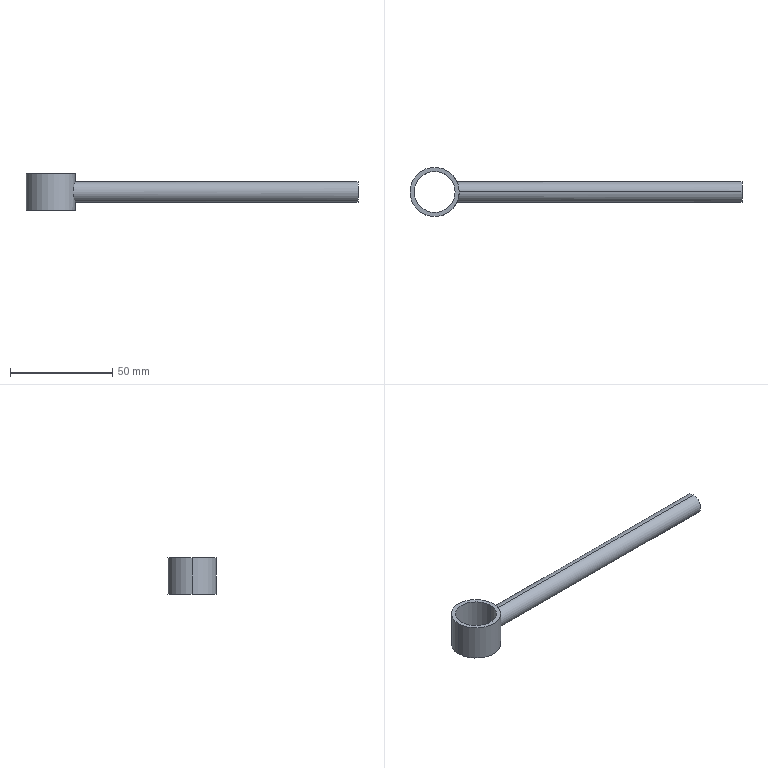Part | SolidWorks | features Extrusion 1, ICE 1 | 1 solid | 9 faces | box 162 x 24 x 18 mm | volume 13348 mm3 | cylinder 6 | plane 3 | commonest cylinder face diameters 10 x2 20 x2 24 x2
STEP:
#1=CARTESIAN_POINT('',(12.,0.,-5.));
#2=VERTEX_POINT('',#1);
#3=CARTESIAN_POINT('',(12.,0.,5.));
#4=VERTEX_POINT('',#3);
#5=CARTESIAN_POINT('',(12.,0.,-5.));
#6=CARTESIAN_POINT('',(12.,0.3345,-5.));
#7=CARTESIAN_POINT('',(11.986,0.6627,-4.967));
#8=CARTESIAN_POINT('',(11.933,1.307,-4.837));
#9=CARTESIAN_POINT('',(11.893,1.627,-4.739));
#10=CARTESIAN_POINT('',(11.795,2.231,-4.487));
#11=CARTESIAN_POINT('',(11.736,2.517,-4.333));
#12=CARTESIAN_POINT('',(11.607,3.058,-3.969));
#13=CARTESIAN_POINT('',(11.537,3.31,-3.761));
#14=CARTESIAN_POINT('',(11.396,3.766,-3.305));
#15=CARTESIAN_POINT('',(11.325,3.972,-3.055));
#16=CARTESIAN_POINT('',(11.191,4.335,-2.512));
#17=CARTESIAN_POINT('',(11.13,4.489,-2.227));
#18=CARTESIAN_POINT('',(11.051,4.677,-1.777));
#19=CARTESIAN_POINT('',(11.028,4.732,-1.623));
#20=CARTESIAN_POINT('',(10.986,4.829,-1.308));
#21=CARTESIAN_POINT('',(10.968,4.87,-1.146));
#22=CARTESIAN_POINT('',(10.924,4.967,-0.6608));
#23=CARTESIAN_POINT('',(10.909,5.,-0.3338));
#24=CARTESIAN_POINT('',(10.909,5.,0.3273));
#25=CARTESIAN_POINT('',(10.924,4.967,0.6627));
#26=CARTESIAN_POINT('',(10.982,4.837,1.308));
#27=CARTESIAN_POINT('',(11.025,4.741,1.622));
#28=CARTESIAN_POINT('',(11.13,4.487,2.231));
#29=CARTESIAN_POINT('',(11.192,4.333,2.516));
#30=CARTESIAN_POINT('',(11.325,3.972,3.054));
#31=CARTESIAN_POINT('',(11.397,3.763,3.308));
#32=CARTESIAN_POINT('',(11.538,3.306,3.765));
#33=CARTESIAN_POINT('',(11.607,3.057,3.97));
#34=CARTESIAN_POINT('',(11.704,2.652,4.242));
#35=CARTESIAN_POINT('',(11.735,2.51,4.327));
#36=CARTESIAN_POINT('',(11.793,2.222,4.482));
#37=CARTESIAN_POINT('',(11.82,2.075,4.552));
#38=CARTESIAN_POINT('',(11.893,1.625,4.74));
#39=CARTESIAN_POINT('',(11.933,1.312,4.836));
#40=CARTESIAN_POINT('',(11.986,0.659,4.968));
#41=CARTESIAN_POINT('',(12.,0.3295,5.));
#42=CARTESIAN_POINT('',(12.,0.,5.));
#43=B_SPLINE_CURVE_WITH_KNOTS('',3,(#5,#6,#7,#8,#9,#10,#11,#12,#13,#14,#15,#16,#17,#18,#19,#20,#21,#22,#23,#24,#25,#26,#27,#28,#29,#30,#31,#32,#33,#34,#35,#36,#37,#38,#39,#40,#41,#42),.UNSPECIFIED.,.F.,.F.,(4,2,2,2,2,2,2,2,2,2,2,2,2,2,2,2,2,2,4),(0.,0.0009884,0.001977,0.002965,0.003954,0.004942,0.005931,0.006425,0.006919,0.007907,0.008896,0.009884,0.01087,0.01186,0.01285,0.01334,0.01384,0.01483,0.01581),.UNSPECIFIED.);
#44=EDGE_CURVE('',#2,#4,#43,.T.);
#45=ORIENTED_EDGE('',*,*,#44,.T.);
#46=CARTESIAN_POINT('',(150.,0.,5.));
#47=VERTEX_POINT('',#46);
#48=CARTESIAN_POINT('',(-12.002,0.,5.));
#49=DIRECTION('',(1.,0.,0.));
#50=VECTOR('',#49,1000.);
#51=LINE('',#48,#50);
#52=EDGE_CURVE('',#4,#47,#51,.T.);
#53=ORIENTED_EDGE('',*,*,#52,.T.);
#54=CARTESIAN_POINT('',(150.,0.,-5.));
#55=VERTEX_POINT('',#54);
#56=CARTESIAN_POINT('',(150.,0.,0.));
#57=DIRECTION('',(1.,0.,0.));
#58=DIRECTION('',(0.,0.,-1.));
#59=AXIS2_PLACEMENT_3D('',#56,#57,#58);
#60=CIRCLE('',#59,5.);
#61=EDGE_CURVE('',#55,#47,#60,.T.);
#62=ORIENTED_EDGE('',*,*,#61,.F.);
#63=CARTESIAN_POINT('',(-12.002,0.,-5.));
#64=DIRECTION('',(1.,0.,0.));
#65=VECTOR('',#64,1000.);
#66=LINE('',#63,#65);
#67=EDGE_CURVE('',#2,#55,#66,.T.);
#68=ORIENTED_EDGE('',*,*,#67,.F.);
#69=EDGE_LOOP('',(#45,#53,#62,#68));
#70=FACE_OUTER_BOUND('',#69,.T.);
#71=CARTESIAN_POINT('',(-12.002,0.,0.));
#72=DIRECTION('',(1.,0.,0.));
#73=DIRECTION('',(0.,0.,-1.));
#74=AXIS2_PLACEMENT_3D('',#71,#72,#73);
#75=CYLINDRICAL_SURFACE('',#74,5.);
#76=ADVANCED_FACE('',(#70),#75,.T.);
#77=CARTESIAN_POINT('',(-10.,0.,9.));
#78=VERTEX_POINT('',#77);
#79=CARTESIAN_POINT('',(10.,0.,9.));
#80=VERTEX_POINT('',#79);
#81=CARTESIAN_POINT('',(0.,0.,9.));
#82=DIRECTION('',(0.,0.,1.));
#83=DIRECTION('',(1.,0.,0.));
#84=AXIS2_PLACEMENT_3D('',#81,#82,#83);
#85=CIRCLE('',#84,10.);
#86=EDGE_CURVE('',#78,#80,#85,.T.);
#87=ORIENTED_EDGE('',*,*,#86,.T.);
#88=CARTESIAN_POINT('',(10.,0.,-9.));
#89=VERTEX_POINT('',#88);
#90=CARTESIAN_POINT('',(10.,0.,9.));
#91=DIRECTION('',(0.,0.,-1.));
#92=VECTOR('',#91,1000.);
#93=LINE('',#90,#92);
#94=EDGE_CURVE('',#80,#89,#93,.T.);
#95=ORIENTED_EDGE('',*,*,#94,.T.);
#96=CARTESIAN_POINT('',(-10.,0.,-9.));
#97=VERTEX_POINT('',#96);
#98=CARTESIAN_POINT('',(0.,0.,-9.));
#99=DIRECTION('',(0.,0.,1.));
#100=DIRECTION('',(1.,0.,0.));
#101=AXIS2_PLACEMENT_3D('',#98,#99,#100);
#102=CIRCLE('',#101,10.);
#103=EDGE_CURVE('',#97,#89,#102,.T.);
#104=ORIENTED_EDGE('',*,*,#103,.F.);
#105=CARTESIAN_POINT('',(-10.,0.,9.));
#106=DIRECTION('',(0.,0.,-1.));
#107=VECTOR('',#106,1000.);
#108=LINE('',#105,#107);
#109=EDGE_CURVE('',#78,#97,#108,.T.);
#110=ORIENTED_EDGE('',*,*,#109,.F.);
#111=EDGE_LOOP('',(#87,#95,#104,#110));
#112=FACE_OUTER_BOUND('',#111,.T.);
#113=CARTESIAN_POINT('',(0.,0.,9.));
#114=DIRECTION('',(0.,0.,-1.));
#115=DIRECTION('',(-1.,0.,0.));
#116=AXIS2_PLACEMENT_3D('',#113,#114,#115);
#117=CYLINDRICAL_SURFACE('',#116,10.);
#118=ADVANCED_FACE('',(#112),#117,.F.);
#119=CARTESIAN_POINT('',(12.,0.,9.));
#120=VERTEX_POINT('',#119);
#121=CARTESIAN_POINT('',(-12.,0.,9.));
#122=VERTEX_POINT('',#121);
#123=CARTESIAN_POINT('',(0.,0.,9.));
#124=DIRECTION('',(0.,0.,1.));
#125=DIRECTION('',(1.,0.,0.));
#126=AXIS2_PLACEMENT_3D('',#123,#124,#125);
#127=CIRCLE('',#126,12.);
#128=EDGE_CURVE('',#120,#122,#127,.T.);
#129=ORIENTED_EDGE('',*,*,#128,.F.);
#130=CARTESIAN_POINT('',(12.,0.,9.));
#131=DIRECTION('',(0.,0.,-1.));
#132=VECTOR('',#131,1000.);
#133=LINE('',#130,#132);
#134=EDGE_CURVE('',#120,#4,#133,.T.);
#135=ORIENTED_EDGE('',*,*,#134,.T.);
#136=ORIENTED_EDGE('',*,*,#44,.F.);
#137=CARTESIAN_POINT('',(12.,0.,-9.));
#138=VERTEX_POINT('',#137);
#139=CARTESIAN_POINT('',(12.,0.,9.));
#140=DIRECTION('',(0.,0.,-1.));
#141=VECTOR('',#140,1000.);
#142=LINE('',#139,#141);
#143=EDGE_CURVE('',#2,#138,#142,.T.);
#144=ORIENTED_EDGE('',*,*,#143,.T.);
#145=CARTESIAN_POINT('',(-12.,0.,-9.));
#146=VERTEX_POINT('',#145);
#147=CARTESIAN_POINT('',(0.,0.,-9.));
#148=DIRECTION('',(0.,0.,1.));
#149=DIRECTION('',(1.,0.,0.));
#150=AXIS2_PLACEMENT_3D('',#147,#148,#149);
#151=CIRCLE('',#150,12.);
#152=EDGE_CURVE('',#138,#146,#151,.T.);
#153=ORIENTED_EDGE('',*,*,#152,.T.);
#154=CARTESIAN_POINT('',(-12.,0.,9.));
#155=DIRECTION('',(0.,0.,-1.));
#156=VECTOR('',#155,1000.);
#157=LINE('',#154,#156);
#158=EDGE_CURVE('',#122,#146,#157,.T.);
#159=ORIENTED_EDGE('',*,*,#158,.F.);
#160=EDGE_LOOP('',(#129,#135,#136,#144,#153,#159));
#161=FACE_OUTER_BOUND('',#160,.T.);
#162=CARTESIAN_POINT('',(0.,0.,9.));
#163=DIRECTION('',(0.,0.,-1.));
#164=DIRECTION('',(-1.,0.,0.));
#165=AXIS2_PLACEMENT_3D('',#162,#163,#164);
#166=CYLINDRICAL_SURFACE('',#165,12.);
#167=ADVANCED_FACE('',(#161),#166,.T.);
#168=CARTESIAN_POINT('',(0.,0.,9.));
#169=DIRECTION('',(0.,0.,1.));
#170=DIRECTION('',(1.,0.,0.));
#171=AXIS2_PLACEMENT_3D('',#168,#169,#170);
#172=CIRCLE('',#171,12.);
#173=EDGE_CURVE('',#122,#120,#172,.T.);
#174=ORIENTED_EDGE('',*,*,#173,.T.);
#175=ORIENTED_EDGE('',*,*,#128,.T.);
#176=EDGE_LOOP('',(#174,#175));
#177=FACE_OUTER_BOUND('',#176,.T.);
#178=ORIENTED_EDGE('',*,*,#86,.F.);
#179=CARTESIAN_POINT('',(0.,0.,9.));
#180=DIRECTION('',(0.,0.,1.));
#181=DIRECTION('',(1.,0.,0.));
#182=AXIS2_PLACEMENT_3D('',#179,#180,#181);
#183=CIRCLE('',#182,10.);
#184=EDGE_CURVE('',#80,#78,#183,.T.);
#185=ORIENTED_EDGE('',*,*,#184,.F.);
#186=EDGE_LOOP('',(#178,#185));
#187=FACE_BOUND('',#186,.T.);
#188=CARTESIAN_POINT('',(0.,0.,9.));
#189=DIRECTION('',(0.,0.,1.));
#190=DIRECTION('',(1.,0.,0.));
#191=AXIS2_PLACEMENT_3D('',#188,#189,#190);
#192=PLANE('',#191);
#193=ADVANCED_FACE('',(#177,#187),#192,.T.);
#194=CARTESIAN_POINT('',(0.,0.,-9.));
#195=DIRECTION('',(0.,0.,1.));
#196=DIRECTION('',(1.,0.,0.));
#197=AXIS2_PLACEMENT_3D('',#194,#195,#196);
#198=CIRCLE('',#197,12.);
#199=EDGE_CURVE('',#146,#138,#198,.T.);
#200=ORIENTED_EDGE('',*,*,#199,.F.);
#201=ORIENTED_EDGE('',*,*,#152,.F.);
#202=EDGE_LOOP('',(#200,#201));
#203=FACE_OUTER_BOUND('',#202,.T.);
#204=ORIENTED_EDGE('',*,*,#103,.T.);
#205=CARTESIAN_POINT('',(0.,0.,-9.));
#206=DIRECTION('',(0.,0.,1.));
#207=DIRECTION('',(1.,0.,0.));
#208=AXIS2_PLACEMENT_3D('',#205,#206,#207);
#209=CIRCLE('',#208,10.);
#210=EDGE_CURVE('',#89,#97,#209,.T.);
#211=ORIENTED_EDGE('',*,*,#210,.T.);
#212=EDGE_LOOP('',(#204,#211));
#213=FACE_BOUND('',#212,.T.);
#214=CARTESIAN_POINT('',(0.,0.,-9.));
#215=DIRECTION('',(0.,0.,1.));
#216=DIRECTION('',(1.,0.,0.));
#217=AXIS2_PLACEMENT_3D('',#214,#215,#216);
#218=PLANE('',#217);
#219=ADVANCED_FACE('',(#203,#213),#218,.F.);
#220=ORIENTED_EDGE('',*,*,#134,.F.);
#221=ORIENTED_EDGE('',*,*,#173,.F.);
#222=ORIENTED_EDGE('',*,*,#158,.T.);
#223=ORIENTED_EDGE('',*,*,#199,.T.);
#224=ORIENTED_EDGE('',*,*,#143,.F.);
#225=CARTESIAN_POINT('',(12.,0.,5.));
#226=CARTESIAN_POINT('',(12.,-0.1646,5.));
#227=CARTESIAN_POINT('',(11.997,-0.3295,4.992));
#228=CARTESIAN_POINT('',(11.983,-0.6596,4.959));
#229=CARTESIAN_POINT('',(11.973,-0.8253,4.934));
#230=CARTESIAN_POINT('',(11.933,-1.311,4.836));
#231=CARTESIAN_POINT('',(11.894,-1.624,4.74));
#232=CARTESIAN_POINT('',(11.82,-2.078,4.551));
#233=CARTESIAN_POINT('',(11.792,-2.228,4.479));
#234=CARTESIAN_POINT('',(11.734,-2.515,4.324));
#235=CARTESIAN_POINT('',(11.704,-2.654,4.24));
#236=CARTESIAN_POINT('',(11.607,-3.057,3.969));
#237=CARTESIAN_POINT('',(11.537,-3.309,3.763));
#238=CARTESIAN_POINT('',(11.395,-3.768,3.302));
#239=CARTESIAN_POINT('',(11.325,-3.973,3.053));
#240=CARTESIAN_POINT('',(11.192,-4.333,2.517));
#241=CARTESIAN_POINT('',(11.129,-4.489,2.226));
#242=CARTESIAN_POINT('',(11.025,-4.741,1.623));
#243=CARTESIAN_POINT('',(10.983,-4.836,1.311));
#244=CARTESIAN_POINT('',(10.924,-4.966,0.6662));
#245=CARTESIAN_POINT('',(10.909,-5.,0.3309));
#246=CARTESIAN_POINT('',(10.909,-5.,-0.3283));
#247=CARTESIAN_POINT('',(10.924,-4.968,-0.6563));
#248=CARTESIAN_POINT('',(10.982,-4.837,-1.309));
#249=CARTESIAN_POINT('',(11.025,-4.741,-1.623));
#250=CARTESIAN_POINT('',(11.129,-4.489,-2.225));
#251=CARTESIAN_POINT('',(11.192,-4.333,-2.516));
#252=CARTESIAN_POINT('',(11.325,-3.972,-3.055));
#253=CARTESIAN_POINT('',(11.396,-3.767,-3.304));
#254=CARTESIAN_POINT('',(11.538,-3.308,-3.763));
#255=CARTESIAN_POINT('',(11.608,-3.055,-3.971));
#256=CARTESIAN_POINT('',(11.736,-2.519,-4.331));
#257=CARTESIAN_POINT('',(11.794,-2.233,-4.486));
#258=CARTESIAN_POINT('',(11.894,-1.623,-4.741));
#259=CARTESIAN_POINT('',(11.933,-1.31,-4.836));
#260=CARTESIAN_POINT('',(11.986,-0.667,-4.966));
#261=CARTESIAN_POINT('',(12.,-0.3342,-5.));
#262=CARTESIAN_POINT('',(12.,0.,-5.));
#263=B_SPLINE_CURVE_WITH_KNOTS('',3,(#225,#226,#227,#228,#229,#230,#231,#232,#233,#234,#235,#236,#237,#238,#239,#240,#241,#242,#243,#244,#245,#246,#247,#248,#249,#250,#251,#252,#253,#254,#255,#256,#257,#258,#259,#260,#261,#262),.UNSPECIFIED.,.F.,.F.,(4,2,2,2,2,2,2,2,2,2,2,2,2,2,2,2,2,2,4),(0.01581,0.01631,0.0168,0.01779,0.01828,0.01878,0.01977,0.02075,0.02174,0.02273,0.02372,0.0247,0.02569,0.02668,0.02767,0.02865,0.02964,0.03063,0.03162),.UNSPECIFIED.);
#264=EDGE_CURVE('',#4,#2,#263,.T.);
#265=ORIENTED_EDGE('',*,*,#264,.F.);
#266=EDGE_LOOP('',(#220,#221,#222,#223,#224,#265));
#267=FACE_OUTER_BOUND('',#266,.T.);
#268=CARTESIAN_POINT('',(0.,0.,9.));
#269=DIRECTION('',(0.,0.,-1.));
#270=DIRECTION('',(-1.,0.,0.));
#271=AXIS2_PLACEMENT_3D('',#268,#269,#270);
#272=CYLINDRICAL_SURFACE('',#271,12.);
#273=ADVANCED_FACE('',(#267),#272,.T.);
#274=ORIENTED_EDGE('',*,*,#94,.F.);
#275=ORIENTED_EDGE('',*,*,#184,.T.);
#276=ORIENTED_EDGE('',*,*,#109,.T.);
#277=ORIENTED_EDGE('',*,*,#210,.F.);
#278=EDGE_LOOP('',(#274,#275,#276,#277));
#279=FACE_OUTER_BOUND('',#278,.T.);
#280=CARTESIAN_POINT('',(0.,0.,9.));
#281=DIRECTION('',(0.,0.,-1.));
#282=DIRECTION('',(-1.,0.,0.));
#283=AXIS2_PLACEMENT_3D('',#280,#281,#282);
#284=CYLINDRICAL_SURFACE('',#283,10.);
#285=ADVANCED_FACE('',(#279),#284,.F.);
#286=ORIENTED_EDGE('',*,*,#52,.F.);
#287=ORIENTED_EDGE('',*,*,#264,.T.);
#288=ORIENTED_EDGE('',*,*,#67,.T.);
#289=CARTESIAN_POINT('',(150.,0.,0.));
#290=DIRECTION('',(1.,0.,0.));
#291=DIRECTION('',(0.,0.,-1.));
#292=AXIS2_PLACEMENT_3D('',#289,#290,#291);
#293=CIRCLE('',#292,5.);
#294=EDGE_CURVE('',#47,#55,#293,.T.);
#295=ORIENTED_EDGE('',*,*,#294,.F.);
#296=EDGE_LOOP('',(#286,#287,#288,#295));
#297=FACE_OUTER_BOUND('',#296,.T.);
#298=CARTESIAN_POINT('',(-12.002,0.,0.));
#299=DIRECTION('',(1.,0.,0.));
#300=DIRECTION('',(0.,0.,-1.));
#301=AXIS2_PLACEMENT_3D('',#298,#299,#300);
#302=CYLINDRICAL_SURFACE('',#301,5.);
#303=ADVANCED_FACE('',(#297),#302,.T.);
#304=ORIENTED_EDGE('',*,*,#61,.T.);
#305=ORIENTED_EDGE('',*,*,#294,.T.);
#306=EDGE_LOOP('',(#304,#305));
#307=FACE_OUTER_BOUND('',#306,.T.);
#308=CARTESIAN_POINT('',(150.,0.,0.));
#309=DIRECTION('',(1.,0.,0.));
#310=DIRECTION('',(0.,0.,-1.));
#311=AXIS2_PLACEMENT_3D('',#308,#309,#310);
#312=PLANE('',#311);
#313=ADVANCED_FACE('',(#307),#312,.T.);
#314=CLOSED_SHELL('',(#76,#118,#167,#193,#219,#273,#285,#303,#313));
#315=MANIFOLD_SOLID_BREP('',#314);
#316=CARTESIAN_POINT('',(0.,0.,0.));
#317=DIRECTION('',(0.,0.,1.));
#318=DIRECTION('',(1.,0.,0.));
#319=AXIS2_PLACEMENT_3D('',#316,#317,#318);
#320=(LENGTH_UNIT()NAMED_UNIT(*)SI_UNIT(.MILLI.,.METRE.));
#321=UNCERTAINTY_MEASURE_WITH_UNIT(LENGTH_MEASURE(0.00001),#320,'','');
#322=(NAMED_UNIT(*)PLANE_ANGLE_UNIT()SI_UNIT($,.RADIAN.));
#323=(NAMED_UNIT(*)SI_UNIT($,.STERADIAN.)SOLID_ANGLE_UNIT());
#324=(GEOMETRIC_REPRESENTATION_CONTEXT(3)GLOBAL_UNCERTAINTY_ASSIGNED_CONTEXT((#321))GLOBAL_UNIT_ASSIGNED_CONTEXT((#320,#322,#323))REPRESENTATION_CONTEXT('',''));
#325=ADVANCED_BREP_SHAPE_REPRESENTATION('',(#315,#319),#324);